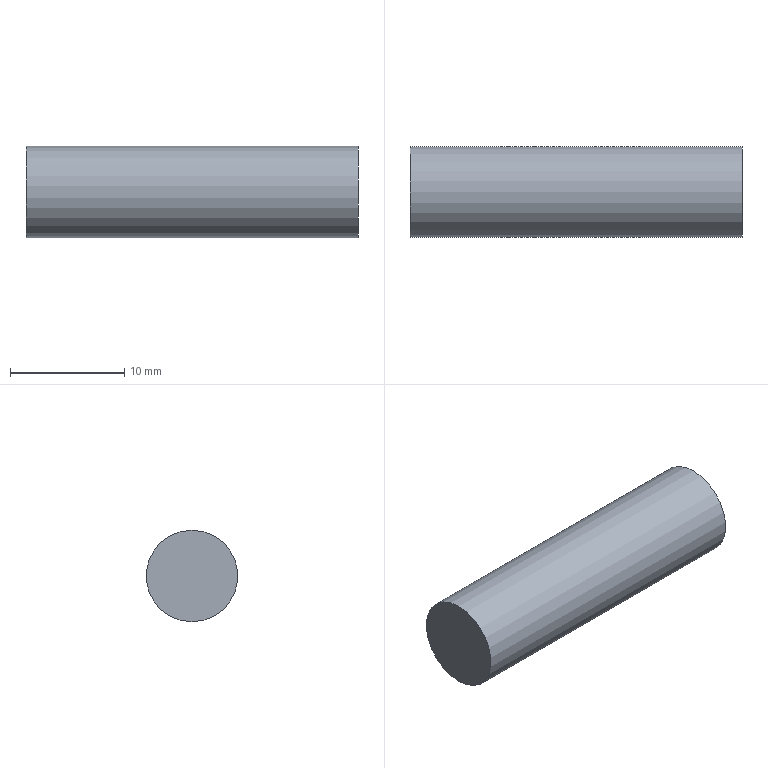Part | STEP file | solid 121 | 1 solid | 3 faces | box 29 x 8 x 8 mm | volume 1458 mm3 | plane 2 | cylinder 1 | commonest cylinder face diameters 8 x1